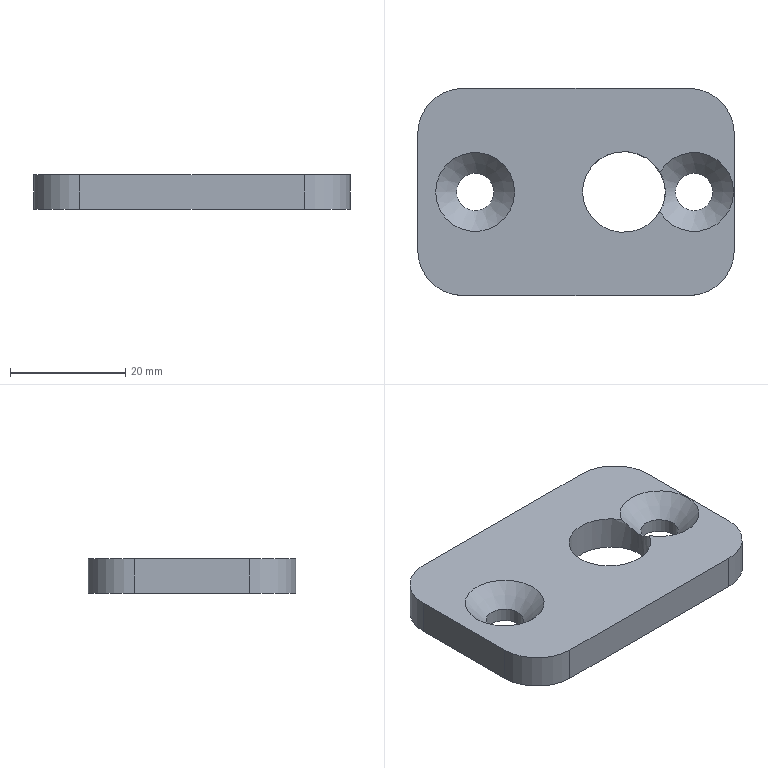Part | STEP file | solid 62 | 1 solid | 15 faces | box 55 x 36 x 6 mm | volume 9848 mm3 | plane 6 | cylinder 6 | cone 2 | other 1 | commonest cylinder face diameters 16 x4 6.5 x2